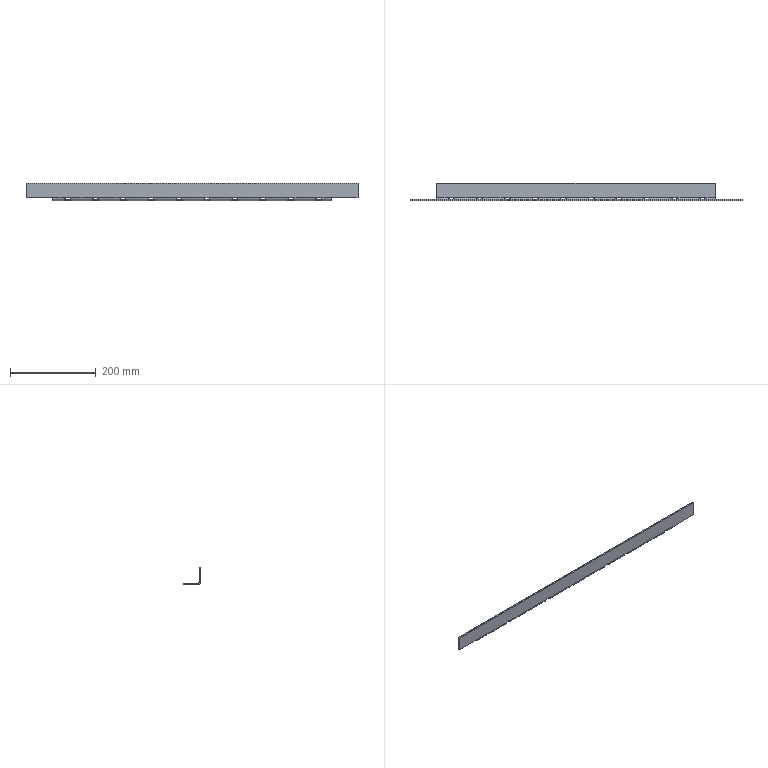Part | NX | features solid 2 | 1 solid | 114 faces | box 775 x 40 x 40 mm | volume 155999 mm3 | cylinder 62 | plane 32 | spline 20 | commonest cylinder face diameters 9 x40 6 x11 12 x11